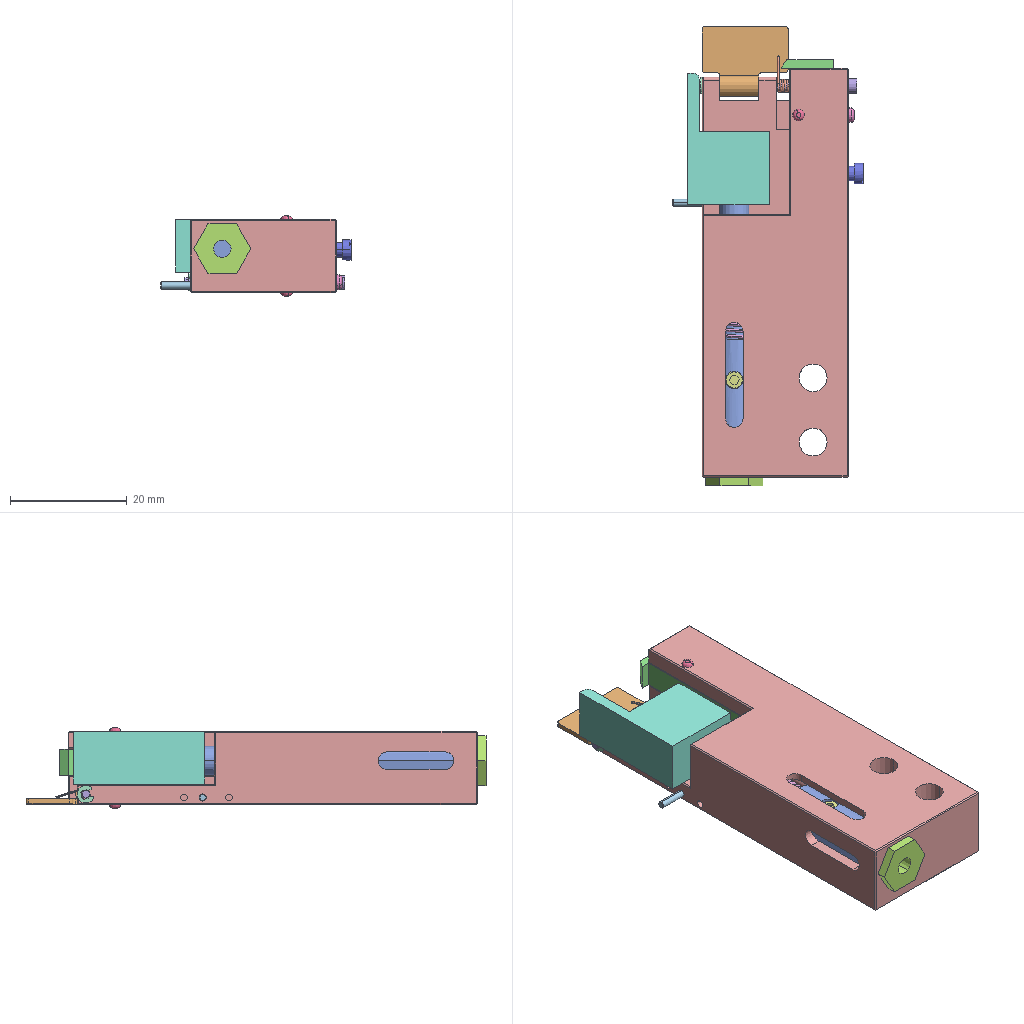Assembly | SolidWorks | 17 different items | 17 placed | box 33 x 79 x 14 mm
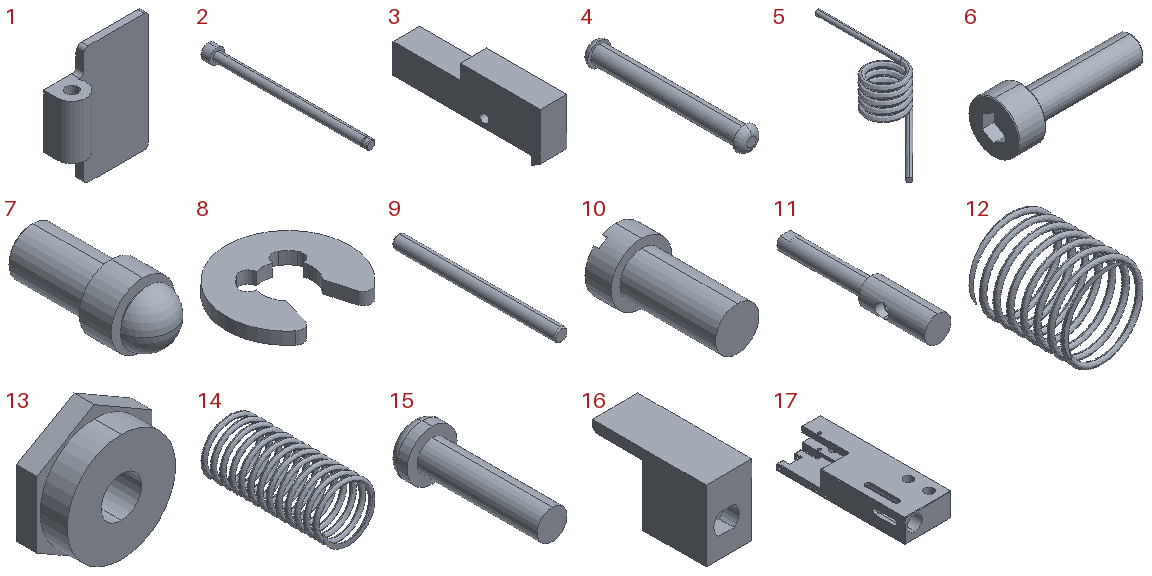Parts list (item | quantity | size | volume | features):
1 | x1 | 12 x 3.5 x 14.7 mm | 181.213 mm3 | features ICE 5, Chamfer 1, Extrusion 1, Fillet 1
2 | x1 | 2.5 x 27.5 x 2.5 mm | 53.096 mm3 | features ICE 2, Chamfer 1, Extrusion 1
3 | x1 | 4.5 x 25 x 9 mm | 714.291 mm3 | features Cut 2, Extrusion 1, ICE 1
4 | x1 | 2 x 13.7 x 2 mm | 25.019 mm3 | features Extrusion 1, Fillet 1, ICE 1, MirrorPattern 1
5 | x1 | 4.085 x 9.349 x 2.35 mm | 2.987 mm3 | features BaseBody 1, ICE 1
6 | x1 | 15 x 5.5 x 5.5 mm | 148.972 mm3 | features BlendCut 1, Chamfer 1, Cut 1, Fillet 1, Revolution 1
7 | x1 | 4 x 8.799 x 4 mm | 69.832 mm3 | features ICE 2, Chamfer 1, Extrusion 1, Revolution 1
8 | x1 | 3 x 2.7 x 0.3 mm | 1.322 mm3 | features Extrusion 1
9 | x1 | 1.2 x 15 x 1.2 mm | 16.929 mm3 | features Chamfer 1, Extrusion 1
10 | x1 | 3.5 x 7 x 3.5 mm | 40.83 mm3 | features Cut 1, Extrusion 1, ICE 1
11 | x1 | 7.9 x 46 x 7.9 mm | 1380 mm3 | features ICE 4, 3DProfileFeature 1, Extrusion 1, HoleWzd 1
12 | x1 | - | 2.155 mm3 | features Helix 1, ICE 1, Sweep 1
13 | x1 | 8.5 x 3.5 x 9.815 mm | 169.646 mm3 | features ICE 2, Extrusion 1
14 | x1 | 6 x 13 x 6 mm | 43.094 mm3 | features Helix 1, ICE 1, Sweep 1
15 | x1 | 2.5 x 7 x 2.5 mm | 14.982 mm3 | features ICE 2, Extrusion 1, Fillet 1
16 | x1 | 9 x 22.5 x 14 mm | 1549 mm3 | features 3DProfileFeature 1, Cut 1, Extrusion 1, Fillet 1, HoleWzd 1, ICE 1
17 | x1 | 25 x 70 x 12.5 mm | 14176 mm3 | features Cut 13, ICE 4, Chamfer 3, Fillet 2, 3DProfileFeature 1, Extrusion 1, HoleWzd 1
Mates (type | each side: item.copy, entity, surface, feature):
Coincident | 17.1 plane | assembly plane | 3 times
Concentric | 17.1 face cylinder Cut-Extrude1 | 11.1 face cylinder Boss-Extrude1
Concentric | 17.1 face cylinder Cut-Extrude1 | 13.1 face cylinder Boss-Extrude1
Coincident | 17.1 face plane Boss-Extrude1 | 13.1 face plane Boss-Extrude2
Parallel | 17.1 face plane Boss-Extrude1 | 13.1 face plane Boss-Extrude2
LimitDistanceDim | 11.1 face plane Boss-Extrude1 | 13.1 face plane Boss-Extrude1
LimitDistanceDim | 11.1 face plane Boss-Extrude1 | 17.1 face plane Cut-Extrude1
Concentric | 11.1 face cylinder Boss-Extrude2 | 14.1 select_type:24
Coincident | 11.1 face plane Boss-Extrude1 | 14.1 face plane Cut-Extrude1
Parallel | 17.1 face plane Boss-Extrude1 | 11.1 plane
Concentric | 11.1 face cylinder Cut-Extrude2 | 7.1 face cylinder Boss-Extrude1
Coincident | 11.1 face plane Cut-Extrude3 | 7.1 face plane Boss-Extrude2
Parallel | 17.1 face plane Cut-Extrude3 | 16.1 face plane Boss-Extrude1
Coincident | 17.1 face plane Cut-Extrude3 | 16.1 face plane Boss-Extrude1
DistanceDim | 16.1 face plane Boss-Extrude1 | 17.1 face plane Boss-Extrude1
Coincident | 11.1 face plane Boss-Extrude2 | 16.1 face plane Cut-Extrude1
Coincident | 16.1 face plane Hole size (per hex socket screw type) 1 | 6.1 face plane Base-Revolve
Concentric | 16.1 face cylinder Hole size (per hex socket screw type) 1 | 6.1 face cylinder Base-Revolve
Parallel | 17.1 face plane Boss-Extrude1 | 1.1 face plane Boss-Extrude1
Width | 1.1 face plane Boss-Extrude1 | 1.1 face plane Boss-Extrude1 | 17.1 face plane Cut-Extrude6 | 17.1 face plane Cut-Extrude6
Concentric | 17.1 face cylinder Cut-Extrude9 | 1.1 face cylinder Boss-Extrude1
Concentric | 17.1 face cylinder Cut-Extrude9 | 2.1 face cylinder Boss-Extrude1
Coincident | 17.1 face plane Boss-Extrude1 | 2.1 face plane Boss-Extrude2
Concentric | 2.1 face cylinder Boss-Extrude1 | 8.1 face cylinder Body
Coincident | 17.1 face plane Boss-Extrude1 | 8.1 face plane Body
Parallel | 17.1 face plane Cut-Extrude3 | 1.1 face plane Boss-Extrude2
Concentric | 2.1 face cylinder Boss-Extrude1 | 5.1 select_type:24
Width | 3.1 face plane Boss-Extrude1 | 3.1 face plane Boss-Extrude1 | 17.1 face plane Cut-Extrude10 | 17.1 face plane Cut-Extrude10
Parallel | 17.1 face plane Cut-Extrude10 | 3.1 face plane Boss-Extrude1
DistanceDim | 17.1 face plane Cut-Extrude10 | 3.1 face plane Boss-Extrude1
DistanceDim | 3.1 face plane Boss-Extrude1 | 17.1 face plane Boss-Extrude1
Concentric | 17.1 face cylinder Cut-Extrude13 | 4.1 face cylinder Boss-Extrude1
Coincident | 17.1 face plane Boss-Extrude1 | 4.1 face plane Boss-Extrude2
Concentric | 17.1 face cylinder Cut-Extrude12 | 9.1 face cylinder Boss-Extrude1
Concentric | 17.1 face cylinder Cut-Extrude16 | 10.1 face cylinder Boss-Extrude1
Concentric | 10.1 face cylinder Boss-Extrude1 | 12.1 select_type:24
Concentric | 17.1 face cylinder Cut-Extrude17 | 15.1 face cylinder Boss-Extrude1
Coincident | 17.1 face plane Boss-Extrude1 | 15.1 face plane Boss-Extrude2